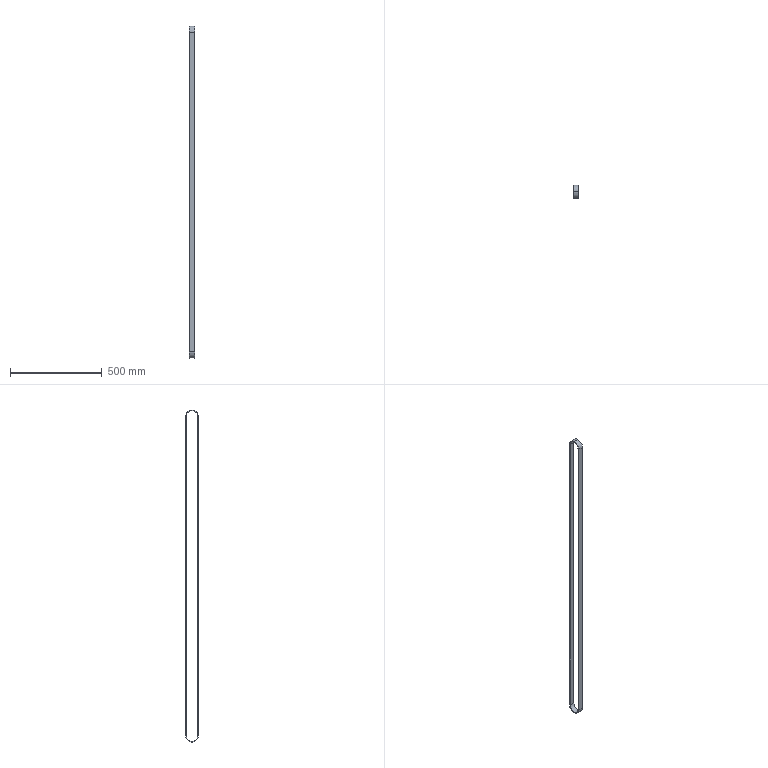Part | SolidWorks | features ExtruThin 1 | 1 solid | 12 faces | box 30 x 70.7 x 1811 mm | volume 497876 mm3 | cylinder 6 | plane 6 | commonest cylinder face diameters 61.7 x3 70.7 x3
STEP:
#1=CARTESIAN_POINT('',(15.,30.85,1740.));
#2=VERTEX_POINT('',#1);
#3=CARTESIAN_POINT('',(15.,0.,1770.85));
#4=VERTEX_POINT('',#3);
#5=CARTESIAN_POINT('',(15.,0.,1740.));
#6=DIRECTION('',(1.,0.,0.));
#7=DIRECTION('',(0.,0.,-1.));
#8=AXIS2_PLACEMENT_3D('',#5,#6,#7);
#9=CIRCLE('',#8,30.85);
#10=EDGE_CURVE('',#2,#4,#9,.T.);
#11=ORIENTED_EDGE('',*,*,#10,.T.);
#12=CARTESIAN_POINT('',(-15.,0.,1770.85));
#13=VERTEX_POINT('',#12);
#14=CARTESIAN_POINT('',(15.,0.,1770.85));
#15=DIRECTION('',(-1.,0.,0.));
#16=VECTOR('',#15,1000.);
#17=LINE('',#14,#16);
#18=EDGE_CURVE('',#4,#13,#17,.T.);
#19=ORIENTED_EDGE('',*,*,#18,.T.);
#20=CARTESIAN_POINT('',(-15.,30.85,1740.));
#21=VERTEX_POINT('',#20);
#22=CARTESIAN_POINT('',(-15.,0.,1740.));
#23=DIRECTION('',(1.,0.,0.));
#24=DIRECTION('',(0.,0.,-1.));
#25=AXIS2_PLACEMENT_3D('',#22,#23,#24);
#26=CIRCLE('',#25,30.85);
#27=EDGE_CURVE('',#21,#13,#26,.T.);
#28=ORIENTED_EDGE('',*,*,#27,.F.);
#29=CARTESIAN_POINT('',(15.,30.85,1740.));
#30=DIRECTION('',(-1.,0.,0.));
#31=VECTOR('',#30,1000.);
#32=LINE('',#29,#31);
#33=EDGE_CURVE('',#2,#21,#32,.T.);
#34=ORIENTED_EDGE('',*,*,#33,.F.);
#35=EDGE_LOOP('',(#11,#19,#28,#34));
#36=FACE_OUTER_BOUND('',#35,.T.);
#37=CARTESIAN_POINT('',(15.,0.,1740.));
#38=DIRECTION('',(-1.,0.,0.));
#39=DIRECTION('',(0.,0.,1.));
#40=AXIS2_PLACEMENT_3D('',#37,#38,#39);
#41=CYLINDRICAL_SURFACE('',#40,30.85);
#42=ADVANCED_FACE('',(#36),#41,.F.);
#43=CARTESIAN_POINT('',(15.,0.,1775.35));
#44=VERTEX_POINT('',#43);
#45=CARTESIAN_POINT('',(15.,-35.35,1740.));
#46=VERTEX_POINT('',#45);
#47=CARTESIAN_POINT('',(15.,0.,1740.));
#48=DIRECTION('',(1.,0.,0.));
#49=DIRECTION('',(0.,0.,-1.));
#50=AXIS2_PLACEMENT_3D('',#47,#48,#49);
#51=CIRCLE('',#50,35.35);
#52=EDGE_CURVE('',#44,#46,#51,.T.);
#53=ORIENTED_EDGE('',*,*,#52,.F.);
#54=CARTESIAN_POINT('',(-15.,0.,1775.35));
#55=VERTEX_POINT('',#54);
#56=CARTESIAN_POINT('',(15.,0.,1775.35));
#57=DIRECTION('',(-1.,0.,0.));
#58=VECTOR('',#57,1000.);
#59=LINE('',#56,#58);
#60=EDGE_CURVE('',#44,#55,#59,.T.);
#61=ORIENTED_EDGE('',*,*,#60,.T.);
#62=CARTESIAN_POINT('',(-15.,-35.35,1740.));
#63=VERTEX_POINT('',#62);
#64=CARTESIAN_POINT('',(-15.,0.,1740.));
#65=DIRECTION('',(1.,0.,0.));
#66=DIRECTION('',(0.,0.,-1.));
#67=AXIS2_PLACEMENT_3D('',#64,#65,#66);
#68=CIRCLE('',#67,35.35);
#69=EDGE_CURVE('',#55,#63,#68,.T.);
#70=ORIENTED_EDGE('',*,*,#69,.T.);
#71=CARTESIAN_POINT('',(15.,-35.35,1740.));
#72=DIRECTION('',(-1.,0.,0.));
#73=VECTOR('',#72,1000.);
#74=LINE('',#71,#73);
#75=EDGE_CURVE('',#46,#63,#74,.T.);
#76=ORIENTED_EDGE('',*,*,#75,.F.);
#77=EDGE_LOOP('',(#53,#61,#70,#76));
#78=FACE_OUTER_BOUND('',#77,.T.);
#79=CARTESIAN_POINT('',(15.,0.,1740.));
#80=DIRECTION('',(-1.,0.,0.));
#81=DIRECTION('',(0.,0.,1.));
#82=AXIS2_PLACEMENT_3D('',#79,#80,#81);
#83=CYLINDRICAL_SURFACE('',#82,35.35);
#84=ADVANCED_FACE('',(#78),#83,.T.);
#85=CARTESIAN_POINT('',(15.,35.35,1740.));
#86=VERTEX_POINT('',#85);
#87=CARTESIAN_POINT('',(15.,0.,1740.));
#88=DIRECTION('',(1.,0.,0.));
#89=DIRECTION('',(0.,0.,-1.));
#90=AXIS2_PLACEMENT_3D('',#87,#88,#89);
#91=CIRCLE('',#90,35.35);
#92=EDGE_CURVE('',#86,#44,#91,.T.);
#93=ORIENTED_EDGE('',*,*,#92,.T.);
#94=ORIENTED_EDGE('',*,*,#52,.T.);
#95=CARTESIAN_POINT('',(15.,-35.35,0.));
#96=VERTEX_POINT('',#95);
#97=CARTESIAN_POINT('',(15.,-35.35,1740.));
#98=DIRECTION('',(0.,0.,-1.));
#99=VECTOR('',#98,1000.);
#100=LINE('',#97,#99);
#101=EDGE_CURVE('',#46,#96,#100,.T.);
#102=ORIENTED_EDGE('',*,*,#101,.T.);
#103=CARTESIAN_POINT('',(15.,35.35,0.));
#104=VERTEX_POINT('',#103);
#105=CARTESIAN_POINT('',(15.,0.,0.));
#106=DIRECTION('',(1.,0.,0.));
#107=DIRECTION('',(0.,0.,-1.));
#108=AXIS2_PLACEMENT_3D('',#105,#106,#107);
#109=CIRCLE('',#108,35.35);
#110=EDGE_CURVE('',#96,#104,#109,.T.);
#111=ORIENTED_EDGE('',*,*,#110,.T.);
#112=CARTESIAN_POINT('',(15.,35.35,0.));
#113=DIRECTION('',(0.,0.,1.));
#114=VECTOR('',#113,1000.);
#115=LINE('',#112,#114);
#116=EDGE_CURVE('',#104,#86,#115,.T.);
#117=ORIENTED_EDGE('',*,*,#116,.T.);
#118=EDGE_LOOP('',(#93,#94,#102,#111,#117));
#119=FACE_OUTER_BOUND('',#118,.T.);
#120=CARTESIAN_POINT('',(15.,-30.85,1740.));
#121=VERTEX_POINT('',#120);
#122=CARTESIAN_POINT('',(15.,-30.85,0.));
#123=VERTEX_POINT('',#122);
#124=CARTESIAN_POINT('',(15.,-30.85,1740.));
#125=DIRECTION('',(0.,0.,-1.));
#126=VECTOR('',#125,1000.);
#127=LINE('',#124,#126);
#128=EDGE_CURVE('',#121,#123,#127,.T.);
#129=ORIENTED_EDGE('',*,*,#128,.F.);
#130=CARTESIAN_POINT('',(15.,0.,1740.));
#131=DIRECTION('',(1.,0.,0.));
#132=DIRECTION('',(0.,0.,-1.));
#133=AXIS2_PLACEMENT_3D('',#130,#131,#132);
#134=CIRCLE('',#133,30.85);
#135=EDGE_CURVE('',#4,#121,#134,.T.);
#136=ORIENTED_EDGE('',*,*,#135,.F.);
#137=ORIENTED_EDGE('',*,*,#10,.F.);
#138=CARTESIAN_POINT('',(15.,30.85,0.));
#139=VERTEX_POINT('',#138);
#140=CARTESIAN_POINT('',(15.,30.85,0.));
#141=DIRECTION('',(0.,0.,1.));
#142=VECTOR('',#141,1000.);
#143=LINE('',#140,#142);
#144=EDGE_CURVE('',#139,#2,#143,.T.);
#145=ORIENTED_EDGE('',*,*,#144,.F.);
#146=CARTESIAN_POINT('',(15.,0.,0.));
#147=DIRECTION('',(1.,0.,0.));
#148=DIRECTION('',(0.,0.,-1.));
#149=AXIS2_PLACEMENT_3D('',#146,#147,#148);
#150=CIRCLE('',#149,30.85);
#151=EDGE_CURVE('',#123,#139,#150,.T.);
#152=ORIENTED_EDGE('',*,*,#151,.F.);
#153=EDGE_LOOP('',(#129,#136,#137,#145,#152));
#154=FACE_BOUND('',#153,.T.);
#155=CARTESIAN_POINT('',(15.,0.,1740.));
#156=DIRECTION('',(1.,0.,0.));
#157=DIRECTION('',(0.,0.,-1.));
#158=AXIS2_PLACEMENT_3D('',#155,#156,#157);
#159=PLANE('',#158);
#160=ADVANCED_FACE('',(#119,#154),#159,.T.);
#161=CARTESIAN_POINT('',(-15.,35.35,1740.));
#162=VERTEX_POINT('',#161);
#163=CARTESIAN_POINT('',(-15.,0.,1740.));
#164=DIRECTION('',(1.,0.,0.));
#165=DIRECTION('',(0.,0.,-1.));
#166=AXIS2_PLACEMENT_3D('',#163,#164,#165);
#167=CIRCLE('',#166,35.35);
#168=EDGE_CURVE('',#162,#55,#167,.T.);
#169=ORIENTED_EDGE('',*,*,#168,.F.);
#170=CARTESIAN_POINT('',(-15.,35.35,0.));
#171=VERTEX_POINT('',#170);
#172=CARTESIAN_POINT('',(-15.,35.35,0.));
#173=DIRECTION('',(0.,0.,1.));
#174=VECTOR('',#173,1000.);
#175=LINE('',#172,#174);
#176=EDGE_CURVE('',#171,#162,#175,.T.);
#177=ORIENTED_EDGE('',*,*,#176,.F.);
#178=CARTESIAN_POINT('',(-15.,-35.35,0.));
#179=VERTEX_POINT('',#178);
#180=CARTESIAN_POINT('',(-15.,0.,0.));
#181=DIRECTION('',(1.,0.,0.));
#182=DIRECTION('',(0.,0.,-1.));
#183=AXIS2_PLACEMENT_3D('',#180,#181,#182);
#184=CIRCLE('',#183,35.35);
#185=EDGE_CURVE('',#179,#171,#184,.T.);
#186=ORIENTED_EDGE('',*,*,#185,.F.);
#187=CARTESIAN_POINT('',(-15.,-35.35,1740.));
#188=DIRECTION('',(0.,0.,-1.));
#189=VECTOR('',#188,1000.);
#190=LINE('',#187,#189);
#191=EDGE_CURVE('',#63,#179,#190,.T.);
#192=ORIENTED_EDGE('',*,*,#191,.F.);
#193=ORIENTED_EDGE('',*,*,#69,.F.);
#194=EDGE_LOOP('',(#169,#177,#186,#192,#193));
#195=FACE_OUTER_BOUND('',#194,.T.);
#196=ORIENTED_EDGE('',*,*,#27,.T.);
#197=CARTESIAN_POINT('',(-15.,-30.85,1740.));
#198=VERTEX_POINT('',#197);
#199=CARTESIAN_POINT('',(-15.,0.,1740.));
#200=DIRECTION('',(1.,0.,0.));
#201=DIRECTION('',(0.,0.,-1.));
#202=AXIS2_PLACEMENT_3D('',#199,#200,#201);
#203=CIRCLE('',#202,30.85);
#204=EDGE_CURVE('',#13,#198,#203,.T.);
#205=ORIENTED_EDGE('',*,*,#204,.T.);
#206=CARTESIAN_POINT('',(-15.,-30.85,0.));
#207=VERTEX_POINT('',#206);
#208=CARTESIAN_POINT('',(-15.,-30.85,1740.));
#209=DIRECTION('',(0.,0.,-1.));
#210=VECTOR('',#209,1000.);
#211=LINE('',#208,#210);
#212=EDGE_CURVE('',#198,#207,#211,.T.);
#213=ORIENTED_EDGE('',*,*,#212,.T.);
#214=CARTESIAN_POINT('',(-15.,30.85,0.));
#215=VERTEX_POINT('',#214);
#216=CARTESIAN_POINT('',(-15.,0.,0.));
#217=DIRECTION('',(1.,0.,0.));
#218=DIRECTION('',(0.,0.,-1.));
#219=AXIS2_PLACEMENT_3D('',#216,#217,#218);
#220=CIRCLE('',#219,30.85);
#221=EDGE_CURVE('',#207,#215,#220,.T.);
#222=ORIENTED_EDGE('',*,*,#221,.T.);
#223=CARTESIAN_POINT('',(-15.,30.85,0.));
#224=DIRECTION('',(0.,0.,1.));
#225=VECTOR('',#224,1000.);
#226=LINE('',#223,#225);
#227=EDGE_CURVE('',#215,#21,#226,.T.);
#228=ORIENTED_EDGE('',*,*,#227,.T.);
#229=EDGE_LOOP('',(#196,#205,#213,#222,#228));
#230=FACE_BOUND('',#229,.T.);
#231=CARTESIAN_POINT('',(-15.,0.,1740.));
#232=DIRECTION('',(1.,0.,0.));
#233=DIRECTION('',(0.,0.,-1.));
#234=AXIS2_PLACEMENT_3D('',#231,#232,#233);
#235=PLANE('',#234);
#236=ADVANCED_FACE('',(#195,#230),#235,.F.);
#237=ORIENTED_EDGE('',*,*,#60,.F.);
#238=ORIENTED_EDGE('',*,*,#92,.F.);
#239=CARTESIAN_POINT('',(15.,35.35,1740.));
#240=DIRECTION('',(-1.,0.,0.));
#241=VECTOR('',#240,1000.);
#242=LINE('',#239,#241);
#243=EDGE_CURVE('',#86,#162,#242,.T.);
#244=ORIENTED_EDGE('',*,*,#243,.T.);
#245=ORIENTED_EDGE('',*,*,#168,.T.);
#246=EDGE_LOOP('',(#237,#238,#244,#245));
#247=FACE_OUTER_BOUND('',#246,.T.);
#248=CARTESIAN_POINT('',(15.,0.,1740.));
#249=DIRECTION('',(-1.,0.,0.));
#250=DIRECTION('',(0.,0.,1.));
#251=AXIS2_PLACEMENT_3D('',#248,#249,#250);
#252=CYLINDRICAL_SURFACE('',#251,35.35);
#253=ADVANCED_FACE('',(#247),#252,.T.);
#254=ORIENTED_EDGE('',*,*,#191,.T.);
#255=CARTESIAN_POINT('',(15.,-35.35,0.));
#256=DIRECTION('',(-1.,0.,0.));
#257=VECTOR('',#256,1000.);
#258=LINE('',#255,#257);
#259=EDGE_CURVE('',#96,#179,#258,.T.);
#260=ORIENTED_EDGE('',*,*,#259,.F.);
#261=ORIENTED_EDGE('',*,*,#101,.F.);
#262=ORIENTED_EDGE('',*,*,#75,.T.);
#263=EDGE_LOOP('',(#254,#260,#261,#262));
#264=FACE_OUTER_BOUND('',#263,.T.);
#265=CARTESIAN_POINT('',(15.,-35.35,1740.));
#266=DIRECTION('',(0.,1.,0.));
#267=DIRECTION('',(0.,0.,1.));
#268=AXIS2_PLACEMENT_3D('',#265,#266,#267);
#269=PLANE('',#268);
#270=ADVANCED_FACE('',(#264),#269,.F.);
#271=ORIENTED_EDGE('',*,*,#185,.T.);
#272=CARTESIAN_POINT('',(15.,35.35,0.));
#273=DIRECTION('',(-1.,0.,0.));
#274=VECTOR('',#273,1000.);
#275=LINE('',#272,#274);
#276=EDGE_CURVE('',#104,#171,#275,.T.);
#277=ORIENTED_EDGE('',*,*,#276,.F.);
#278=ORIENTED_EDGE('',*,*,#110,.F.);
#279=ORIENTED_EDGE('',*,*,#259,.T.);
#280=EDGE_LOOP('',(#271,#277,#278,#279));
#281=FACE_OUTER_BOUND('',#280,.T.);
#282=CARTESIAN_POINT('',(15.,0.,0.));
#283=DIRECTION('',(-1.,0.,0.));
#284=DIRECTION('',(0.,0.,1.));
#285=AXIS2_PLACEMENT_3D('',#282,#283,#284);
#286=CYLINDRICAL_SURFACE('',#285,35.35);
#287=ADVANCED_FACE('',(#281),#286,.T.);
#288=ORIENTED_EDGE('',*,*,#176,.T.);
#289=ORIENTED_EDGE('',*,*,#243,.F.);
#290=ORIENTED_EDGE('',*,*,#116,.F.);
#291=ORIENTED_EDGE('',*,*,#276,.T.);
#292=EDGE_LOOP('',(#288,#289,#290,#291));
#293=FACE_OUTER_BOUND('',#292,.T.);
#294=CARTESIAN_POINT('',(15.,35.35,0.));
#295=DIRECTION('',(0.,-1.,0.));
#296=DIRECTION('',(0.,0.,-1.));
#297=AXIS2_PLACEMENT_3D('',#294,#295,#296);
#298=PLANE('',#297);
#299=ADVANCED_FACE('',(#293),#298,.F.);
#300=ORIENTED_EDGE('',*,*,#18,.F.);
#301=ORIENTED_EDGE('',*,*,#135,.T.);
#302=CARTESIAN_POINT('',(15.,-30.85,1740.));
#303=DIRECTION('',(-1.,0.,0.));
#304=VECTOR('',#303,1000.);
#305=LINE('',#302,#304);
#306=EDGE_CURVE('',#121,#198,#305,.T.);
#307=ORIENTED_EDGE('',*,*,#306,.T.);
#308=ORIENTED_EDGE('',*,*,#204,.F.);
#309=EDGE_LOOP('',(#300,#301,#307,#308));
#310=FACE_OUTER_BOUND('',#309,.T.);
#311=CARTESIAN_POINT('',(15.,0.,1740.));
#312=DIRECTION('',(-1.,0.,0.));
#313=DIRECTION('',(0.,0.,1.));
#314=AXIS2_PLACEMENT_3D('',#311,#312,#313);
#315=CYLINDRICAL_SURFACE('',#314,30.85);
#316=ADVANCED_FACE('',(#310),#315,.F.);
#317=ORIENTED_EDGE('',*,*,#212,.F.);
#318=ORIENTED_EDGE('',*,*,#306,.F.);
#319=ORIENTED_EDGE('',*,*,#128,.T.);
#320=CARTESIAN_POINT('',(15.,-30.85,0.));
#321=DIRECTION('',(-1.,0.,0.));
#322=VECTOR('',#321,1000.);
#323=LINE('',#320,#322);
#324=EDGE_CURVE('',#123,#207,#323,.T.);
#325=ORIENTED_EDGE('',*,*,#324,.T.);
#326=EDGE_LOOP('',(#317,#318,#319,#325));
#327=FACE_OUTER_BOUND('',#326,.T.);
#328=CARTESIAN_POINT('',(15.,-30.85,1740.));
#329=DIRECTION('',(0.,1.,0.));
#330=DIRECTION('',(0.,0.,1.));
#331=AXIS2_PLACEMENT_3D('',#328,#329,#330);
#332=PLANE('',#331);
#333=ADVANCED_FACE('',(#327),#332,.T.);
#334=ORIENTED_EDGE('',*,*,#221,.F.);
#335=ORIENTED_EDGE('',*,*,#324,.F.);
#336=ORIENTED_EDGE('',*,*,#151,.T.);
#337=CARTESIAN_POINT('',(15.,30.85,0.));
#338=DIRECTION('',(-1.,0.,0.));
#339=VECTOR('',#338,1000.);
#340=LINE('',#337,#339);
#341=EDGE_CURVE('',#139,#215,#340,.T.);
#342=ORIENTED_EDGE('',*,*,#341,.T.);
#343=EDGE_LOOP('',(#334,#335,#336,#342));
#344=FACE_OUTER_BOUND('',#343,.T.);
#345=CARTESIAN_POINT('',(15.,0.,0.));
#346=DIRECTION('',(-1.,0.,0.));
#347=DIRECTION('',(0.,0.,1.));
#348=AXIS2_PLACEMENT_3D('',#345,#346,#347);
#349=CYLINDRICAL_SURFACE('',#348,30.85);
#350=ADVANCED_FACE('',(#344),#349,.F.);
#351=ORIENTED_EDGE('',*,*,#227,.F.);
#352=ORIENTED_EDGE('',*,*,#341,.F.);
#353=ORIENTED_EDGE('',*,*,#144,.T.);
#354=ORIENTED_EDGE('',*,*,#33,.T.);
#355=EDGE_LOOP('',(#351,#352,#353,#354));
#356=FACE_OUTER_BOUND('',#355,.T.);
#357=CARTESIAN_POINT('',(15.,30.85,0.));
#358=DIRECTION('',(0.,-1.,0.));
#359=DIRECTION('',(0.,0.,-1.));
#360=AXIS2_PLACEMENT_3D('',#357,#358,#359);
#361=PLANE('',#360);
#362=ADVANCED_FACE('',(#356),#361,.T.);
#363=CLOSED_SHELL('',(#42,#84,#160,#236,#253,#270,#287,#299,#316,#333,#350,#362));
#364=MANIFOLD_SOLID_BREP('',#363);
#365=CARTESIAN_POINT('',(0.,0.,0.));
#366=DIRECTION('',(0.,0.,1.));
#367=DIRECTION('',(1.,0.,0.));
#368=AXIS2_PLACEMENT_3D('',#365,#366,#367);
#369=(LENGTH_UNIT()NAMED_UNIT(*)SI_UNIT(.MILLI.,.METRE.));
#370=UNCERTAINTY_MEASURE_WITH_UNIT(LENGTH_MEASURE(0.00001),#369,'','');
#371=(NAMED_UNIT(*)PLANE_ANGLE_UNIT()SI_UNIT($,.RADIAN.));
#372=(NAMED_UNIT(*)SI_UNIT($,.STERADIAN.)SOLID_ANGLE_UNIT());
#373=(GEOMETRIC_REPRESENTATION_CONTEXT(3)GLOBAL_UNCERTAINTY_ASSIGNED_CONTEXT((#370))GLOBAL_UNIT_ASSIGNED_CONTEXT((#369,#371,#372))REPRESENTATION_CONTEXT('',''));
#374=ADVANCED_BREP_SHAPE_REPRESENTATION('',(#364,#368),#373);